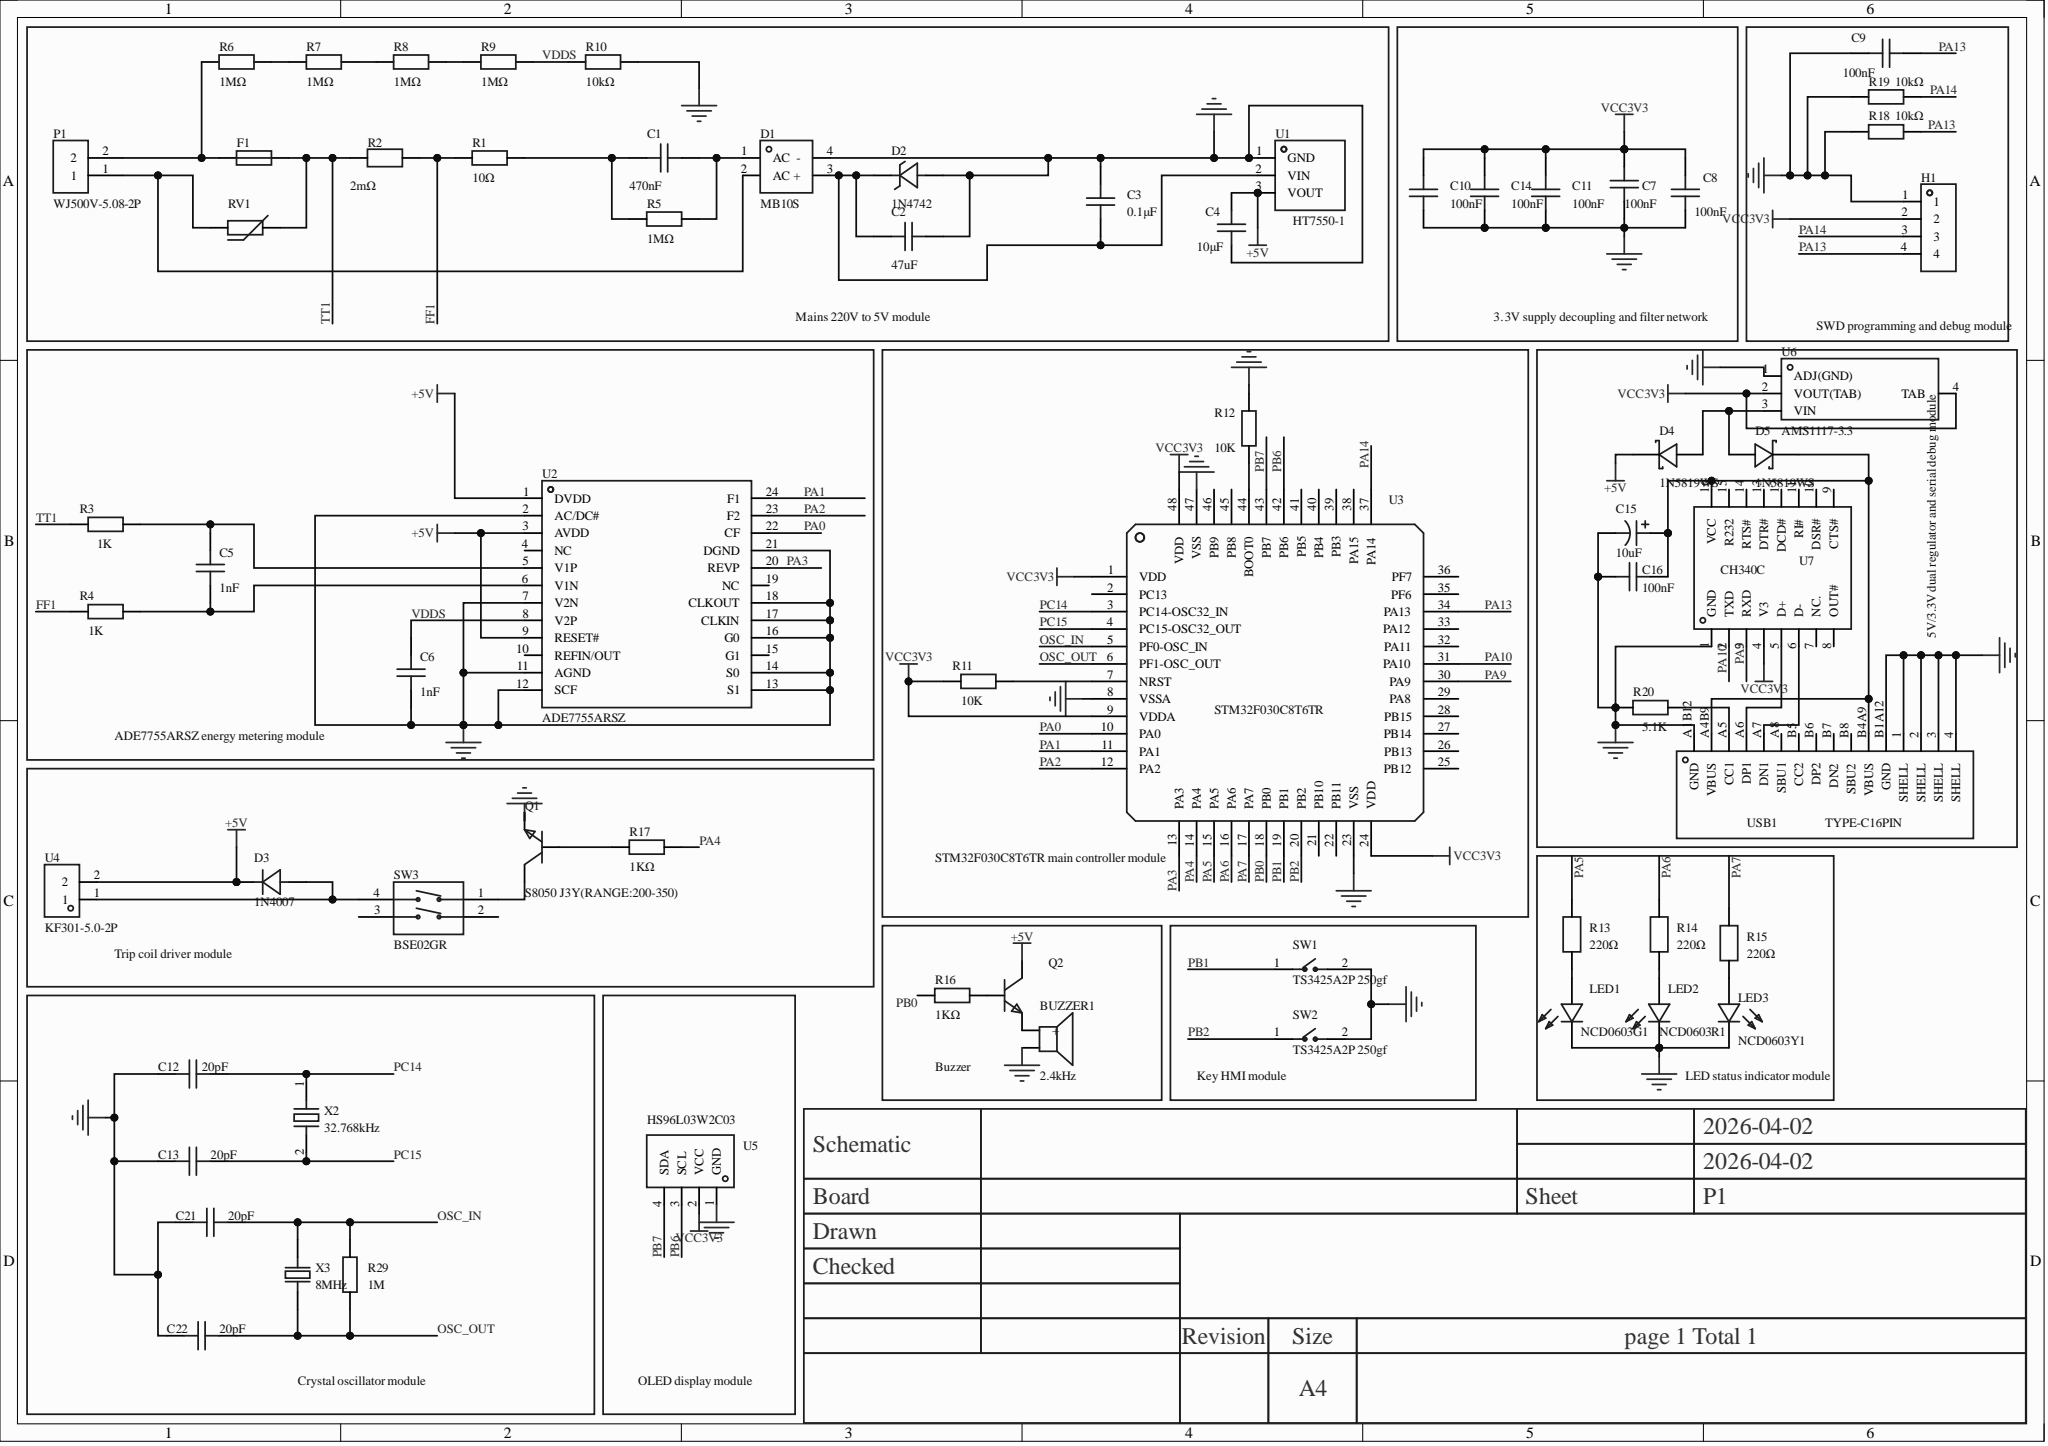Circuit board | Altium Designer | 67 parts | 52 nets
Bill of materials:
Comment,Description,Designator,Footprint,LibRef,Quantity
"2.4kHz","Drive method: Active (with built-in driver circuit); Construction type: Electromagnetic; Rated voltage: 5V; Frequency: 2.4kHz; Sound pressure (SPL): 85dB;","BUZZER1","BUZ-TH_BD12.0-P7.60-D0.6-FD","TMB12A05_C96093","1"
"470nF","Capacitance: 470nF; Tolerance: ±5%; Rated voltage: 400V; Operating temperature: -40℃~+105℃;","C1","CAP-TH_L17.0-W5.5-P15.00-D1.2","CBB21-400V474JP15","1"
"47uF","Capacitance: 47uF; Tolerance: ±20%; Rated voltage: 6.3V; Temperature coefficient: X5R;","C2","C0603","CL10A476MQ8QRNC","1"
"0.1µF","","C3","C0603","CAP_0603","1"
"10µF","","C4","C0603","CAP_0603","1"
"1nF","","C5, C6","C0603","CAP_0603","2"
"100nF","Capacitance: 100nF; Tolerance: ±10%; Rated voltage: 50V; Temperature coefficient: X7R;","C7, C8, C10, C14","C0805","GRM21BR71H104KA01L","4"
"100nF","Capacitance: 100nF; Tolerance: ±10%; Rated voltage: 50V; Temperature coefficient: X7R;, [NoValue]","C9, C11, C16","C0603","FCC0603B104K500CT, CAP_0603, CGA0603X7R104K500JT","3"
"20pF","","C12, C13, C21, C22","C0805","CAP_0805","4"
"10uF","Capacitance: 10uF; Tolerance: ±20%; Rated voltage: 50V; Ripple current: 24mA@120Hz; Equivalent series resistance (ESR): -;","C15","CAP-SMD_BD5.0-L5.3-W5.3-FD","RST10UF50V016","1"
"MB10S","Forward voltage (Vf): 1.1V@1A; DC reverse voltage (Vr): 1kV; Rectified current: 1A; Non-repetitive peak surge current (Ifsm): 35A;","D1","MBS_L4.7-W4.0-P2.50-LS7.0-TL","MB10S_C42463381","1"
"1N4742","Diode configuration: Single; Zener voltage (nominal): 12V; Zener voltage (range): 11.45V~12.95V; Power dissipation (Pd): 1W;","D2","DO-41_BD2.4-L4.7-P8.70-D0.8-FD","1N4742","1"
"1N4007","Diode configuration: Single; Forward voltage (Vf): 1.1V@1A; DC reverse voltage (Vr): 1kV; Rectified current: 1A;","D3","SMA_L4.3-W2.5-LS5.0-RD","1N4007_C727081","1"
"1N5819WS","Forward voltage (Vf): 600mV@1A; DC reverse voltage (Vr): 40V; Rectified current: 1A;","D4, D5","SOD-323_L1.8-W1.3-LS2.5-RD","1N5819WS_C191023","2"
"2F0.05002S1B02","Type: glass tube fuse; Rated current: 500mA; Rated voltage (AC): 250V; 125V; Breaking capacity: 50A;","F1","FUSE-TH_BD3.0-L7.2-P11.20-D0.6","2F0.05002S1B02","1"
"","","H1","HDR-TH_4P-P2.54-V-F","HDR-F_2.54_1x4P","1"
"NCD0603G1","Lamp head type: -; Emitting color: Emerald green; Forward voltage (Vf): 2.6V~3.6V; Power: 72mW; Forward current: 20mA; Wavelength: 515nm~530nm; Diode configuration: Single diode; Lens color: -; Color temperature: -; Luminous intensity: 900mcd; Viewing angle: 130°; Tape packing: -; Operating temperature: -30℃~+85℃;","LED1","LED0603-RD_1","NCD0603G1","1"
"NCD0603R1","Lamp head type: -; Emitting color: Red; Forward voltage (Vf): 1.6V~2.6V; Power: 65mW; Forward current: 25mA; Wavelength: 615nm~630nm; Diode configuration: Single diode; Lens color: -; Color temperature: -; Luminous intensity: 220mcd; Viewing angle: 130°; Tape packing: -; Operating temperature: -30℃~+85℃;","LED2","LED0603-RD_RED","NCD0603R1_C84263","1"
"NCD0603Y1","Lamp head type: -; Emitting color: Yellow; Forward voltage (Vf): 1.6V~2.6V; Power: 65mW; Forward current: 25mA; Wavelength: 586nm~595nm; Diode configuration: Single diode; Lens color: -; Color temperature: -; Luminous intensity: 220mcd; Viewing angle: 130°; Tape packing: -; Operating temperature: -30℃~+85℃;","LED3","LED0603-RD","NCD0603Y1","1"
"WJ500V-5.08-2P","Structure: 1x2P; Pitch: 5.08mm; Color: Green; Mounting: Through-hole; Rated current: 18A; Rated voltage: 250V; Rows: 1; Wire gauge - AWG: 14~30; Wire gauge - mm²: 2.5; Pins per row: 2; Contact material: -; Contact plating: -; Operating temperature range: -40℃~+105℃; Soldering temperature (max.): -;","P1","CONN-TH_2P-P5.00_WJ500V-5.08-2P","WJ500V-5.08-2P","1"
"S8050 J3Y(RANGE:200-350)","Transistor type: NPN; Collector current (Ic): 500mA; Collector-emitter breakdown voltage (Vceo): 25V; Power dissipation (Pd): 300mW; DC current gain (hFE): 200@500mA,1V;","Q1","SOT-23-3_L3.0-W1.7-P0.95-LS2.9-BR","S8050 J3Y(RANGE:200-350)","1"
"","","Q2","S8050_SOT-23","S8050_SOT_NPN","1"
"10Ω","","R1","R0603","Res_0603","1"
"2mΩ","Resistor type: Sense resistor; Resistance: 2mΩ; Tolerance: ±1%; Rated voltage drop: -; Power: 3W; Temperature coefficient: ±50ppm/?; Mounting: SMD;","R2","RES-SMD_L6.4-W3.2-1","HoLLR2512-3W-2mR-1%","1"
"1K","","R3, R4","R0603","Res_0603","2"
"1MΩ","","R5","R0603","Res_0603","1"
"1MΩ","Resistor type: Thick-film resistor; Resistance: 1MΩ; Tolerance: ±1%; Power: 250mW; Operating voltage: 200V; Temperature coefficient: ±100ppm/?;","R6, R7, R8, R9","R1206","1206W4F1004T5E","4"
"10kΩ","Resistor type: Thick-film resistor; Resistance: 10kΩ; Tolerance: ±1%; Power: 125mW; Operating voltage: 150V; Temperature coefficient: ±100ppm/?;","R10, R18, R19","R0805","0805W8F1002T5E_C17414","3"
"10K","","R11, R12","R0603","Res_0603","2"
"220Ω","Resistor type: Thick-film resistor; Resistance: 220Ω; Tolerance: ±1%; Power: 62.5mW; Operating voltage: 50V; Temperature coefficient: ±100ppm/?;","R13, R14, R15","R0402","FRC0402F2200TS","3"
"1KΩ","","R16, R17","R0603","Res_0603","2"
"5.1K","","R20","R0603","Res_0603","1"
"1M","","R29","R0805","Res_0805","1"
"190pF@1kHz","Varistor voltage: 423V~517V; Clamping voltage: 775V; Operating voltage (DC): 385V; Operating voltage (AC): 300V;","RV1","RES-TH_L12.5-W6.7-P7.50-D1.2","10D471K_C8760","1"
"TS3425A2P 250gf","Circuit structure: SPST; Button shape: Round; Actuation force: 2.5N; Mounting: Upright SMD; Length: 3.9mm; Width: 2.9mm; Height: 2.5mm; Bracket: No bracket; Contact current: 50mA; Rated voltage: 12V; Lamp: None; Operating life: 5 ten-thousand cycles;","SW1, SW2","SW-SMD_L3.9-W2.9-LS5.0","TS3425A2P 250gf","2"
"BSE02GR","Circuit structure: SPST; Number of positions: 2; Rated current: 25mA; Rated voltage: 24V; Operating life: 2 thousand cycles; Color: Red;","SW3","SW-TH_4P-L9.9-W6.8-P7.62-BL","BSE02GR","1"
"HT7550-1","Output type: Fixed; Operating voltage: 30V; Output voltage: 5V; Output current: 100mA; Power supply rejection ratio (PSRR): -; Output polarity: Positive;","U1","SOT-89_L4.5-W2.5-P1.50-LS4.2-BR","HT7550-1_C347189","1"
"ADE7755ARSZ","Operating voltage: 4.75V~5.25V; Operating current: 3.5mA;","U2","SSOP-24_L8.1-W5.3-P0.65-LS7.8-BL","ADE7755ARSZ","1"
"STM32F030C8T6TR","CPU core: ARM-M0; CPU max. frequency: 48MHz; Application field: -;","U3","LQFP-48_L7.0-W7.0-P0.50-LS9.0-BL","STM32F030C8T6TR","1"
"KF301-5.0-2P","Structure: 1x2P; Pitch: 5mm; Color: Blue; Mounting: Through-hole; Rows: 1; Pins per row: 2; Rated current: 17A; Rated voltage: 250V; Wire gauge - AWG: 14~22; Wire gauge - mm²: 1.5; Operating temperature: -30℃~+120℃;","U4","HDR-M-2.54_1X2","KF301-5.0-2P","1"
"HS96L03W2C03","Core chip: SSD1315 chip; Interface type: I2C; Size (inch): 0.96; Pixel resolution: 128x64;","U5","OLED-TH_L27.8-W27.2-P2.54_C9900033791","HS96L03W2C03","1"
"AMS1117-3.3","Output type: Fixed; Operating voltage: 12V; Output voltage: 3.3V; Output current: 1A; Power supply rejection ratio (PSRR): 60dB@(120Hz); Output polarity: Positive;","U6","SOT-223-4_L6.5-W3.5-P2.30-LS7.0-BR","AMS1117-3.3_C347222","1"
"CH340C","Application function: Transceiver; USB protocol version: USB 2.0; Data rate: 2Mbps;","U7","SOP-16_L10.0-W3.9-P1.27-LS6.0-BL","CH340C","1"
"TYPE-C16PIN","Connector type: Type-C; Protocol standard: -; Gender: Female; Mounting: Flat SMD; Contact count: 16P; Port count: 1; Rated current - power: 3A; Operating temperature: -40℃~+85℃;","USB1","USB-C-SMD_TYPE-C16PIN","TYPE-C16PIN","1"
"32.768kHz","Crystal type: SMD crystal; Frequency: 32.768kHz; Room-temperature frequency deviation: ±20ppm; Load capacitance: 20pF;","X2","CRYSTAL-SMD_L3.2-W1.5-FC-135R32.768KF-A3","7LC32768F06UC","1"
"8MHz","Crystal type: SMD crystal; Frequency: 8MHz; Room-temperature frequency deviation: ±10ppm; Load capacitance: 12pF; Frequency stability: ±20ppm;","X3","CRYSTAL-SMD_L3.2-W2.5_3225-8MHZ","X22EL89COI-111YLC-8M","1"
Netlist (Protel format):
[
BUZZER1
BUZ-TH_BD12.0-P7.60-D0.6-FD
2.4kHz



]
[
C1
CAP-TH_L17.0-W5.5-P15.00-D1.2
470nF



]
[
C2
C0603
47uF



]
[
C3
C0603
0.1µF



]
[
C4
C0603
10µF



]
[
C5
C0603
1nF



]
[
C6
C0603
1nF



]
[
C7
C0805
100nF



]
[
C8
C0805
100nF



]
[
C9
C0603
100nF



]
[
C10
C0805
100nF



]
[
C11
C0603
100nF



]
[
C12
C0805
20pF



]
[
C13
C0805
20pF



]
[
C14
C0805
100nF



]
[
C15
CAP-SMD_BD5.0-L5.3-W5.3-FD
10uF



]
[
C16
C0603
100nF



]
[
C21
C0805
20pF



]
[
C22
C0805
20pF



]
[
D1
MBS_L4.7-W4.0-P2.50-LS7.0-TL
MB10S



]
[
D2
DO-41_BD2.4-L4.7-P8.70-D0.8-FD
1N4742



]
[
D3
SMA_L4.3-W2.5-LS5.0-RD
1N4007



]
[
D4
SOD-323_L1.8-W1.3-LS2.5-RD
1N5819WS



]
[
D5
SOD-323_L1.8-W1.3-LS2.5-RD
1N5819WS



]
[
F1
FUSE-TH_BD3.0-L7.2-P11.20-D0.6
2F.0500212000S1B02



]
[
H1
HDR-TH_4P-P2.54-V-F




]
[
LED1
LED0603-RD_1
NCD0603G1



]
[
LED2
LED0603-RD_RED
NCD0603R1



]
[
LED3
LED0603-RD
NCD0603Y1



]
[
P1
CONN-TH_2P-P5.00_WJ500V-5.08-2P
WJ500V-5.08-2P



]
[
Q1
SOT-23-3_L3.0-W1.7-P0.95-LS2.9-BR
S8050 J3Y(RANGE:200-350)



]
[
Q2
S8050_SOT-23




]
[
R1
R0603
10Ω



]
[
R2
RES-SMD_L6.4-W3.2-1
2mΩ



]
[
R3
R0603
1K



]
[
R4
R0603
1K



]
[
R5
R0603
1MΩ



]
[
R6
R1206
1MΩ



]
[
R7
R1206
1MΩ



]
[
R8
R1206
1MΩ



]
[
R9
R1206
1MΩ



]
[
R10
R0805
10kΩ



]
[
R11
R0603
10K



]
[
R12
R0603
10K



]
[
R13
R0402
220Ω



]
[
R14
R0402
220Ω



]
[
R15
R0402
220Ω



]
[
R16
R0603
1KΩ



]
[
R17
R0603
1KΩ



]
[
R18
R0805
10kΩ



]
[
R19
R0805
10kΩ



]
[
R20
R0603
5.1K



]
[
R29
R0805
1M



]
[
RV1
RES-TH_L12.5-W6.7-P7.50-D1.2
190pF@1kHz



]
[
SW1
SW-SMD_L3.9-W2.9-LS5.0
TS3425A2P 250gf



]
[
SW2
SW-SMD_L3.9-W2.9-LS5.0
TS3425A2P 250gf



]
[
SW3
SW-TH_4P-L9.9-W6.8-P7.62-BL
BSE02GR



]
[
U1
SOT-89_L4.5-W2.5-P1.50-LS4.2-BR
HT7550-1



]
[
U2
SSOP-24_L8.1-W5.3-P0.65-LS7.8-BL
ADE7755ARSZ



]
[
U3
LQFP-48_L7.0-W7.0-P0.50-LS9.0-BL
STM32F030C8T6TR



]
[
U4
HDR-M-2.54_1X2
KF301-5.0-2P



]
[
U5
OLED-TH_L27.8-W27.2-P2.54_C9900033791
HS96L03W2C03



]
[
U6
SOT-223-4_L6.5-W3.5-P2.30-LS7.0-BR
AMS1117-3.3



]
[
U7
SOP-16_L10.0-W3.9-P1.27-LS6.0-BL
CH340C



]
[
USB1
USB-C-SMD_TYPE-C16PIN
TYPE-C16PIN



]
[
X2
CRYSTAL-SMD_L3.2-W1.5-FC-135R32.7680KF-A3
32.768kHz



]
[
X3
CRYSTAL-SMD_L3.2-W2.5_3225-8MHZ
8MHz



]
(
VDDS
C6-2
R9-2
R10-1
U2-8
)
(
VCC3V3
C7-1
C8-2
C10-1
C11-2
C14-2
H1-2
R11-1
U3-1
U3-9
U3-24
U3-48
U5-2
U6-2
U6-4
U7-4
)
(
TT1
F1-2
R2-1
R3-1
RV1-2
)
(
PC15
C13-2
U3-4
X2-2
)
(
PC14
C12-1
U3-3
X2-1
)
(
PB7
U3-43
U5-4
)
(
PB6
U3-42
U5-3
)
(
PB2
SW2-1
U3-20
)
(
PB1
SW1-1
U3-19
)
(
PB0
R16-2
U3-18
)
(
PA14
H1-3
R19-1
U3-37
)
(
PA13
C9-2
H1-4
R18-1
U3-34
)
(
PA10
U3-31
U7-2
)
(
PA9
U3-30
U7-3
)
(
PA7
R15-2
U3-17
)
(
PA6
R14-2
U3-16
)
(
PA5
R13-2
U3-15
)
(
PA4
R17-1
U3-14
)
(
PA3
U2-20
U3-13
)
(
PA2
U2-23
U3-12
)
(
PA1
U2-24
U3-11
)
(
PA0
U2-22
U3-10
)
(
OSC_OUT
C22-2
R29-1
U3-6
X3-1
)
(
OSC_IN
C21-2
R29-2
U3-5
X3-2
)
(
NetU7_6
U7-6
USB1-A7
)
(
NetU7_5
U7-5
USB1-A6
)
(
NetR20_1
R20-1
USB1-A5
)
(
NetR12_1
R12-1
U3-44
)
(
NetR11_2
R11-2
U3-7
)
(
NetR8_2
R8-2
R9-1
)
(
NetR7_2
R7-2
R8-1
)
(
NetR6_2
R6-2
R7-1
)
(
NetQ2_1
Q2-1
R16-1
)
(
NetQ1_3
Q1-3
SW3-1
)
(
NetQ1_1
Q1-1
R17-2
)
(
NetLED3_2
LED3-2
R15-1
)
(
NetLED2_2
LED2-2
R14-1
)
(
NetLED1_2
LED1-2
R13-1
)
(
NetF1_1
F1-1
P1-2
R6-1
)
(
NetD4_2
D4-2
D5-2
U6-3
)
(
NetD3_2
D3-2
SW3-4
U4-1
)
(
NetD1_2
D1-2
P1-1
RV1-1
)
(
NetC15_1
C15-1
C16-2
D5-1
U7-16
USB1-A4B9
USB1-B4A9
)
(
NetC5_2
C5-2
R3-2
U2-5
)
(
NetC5_1
C5-1
R4-2
U2-6
)
(
NetC2_1
C2-1
C3-1
D1-3
D2-2
U1-2
)
(
NetC1_2
C1-2
R1-2
R5-1
)
(
NetC1_1
C1-1
D1-1
R5-2
)
(
NetBUZZER1_1
BUZZER1-1
Q2-2
)
(
GND
BUZZER1-2
C2-2
C3-2
C4-1
C6-1
C7-2
C8-1
C9-1
C10-2
C11-1
C12-2
C13-1
C14-1
C15-2
C16-1
C21-1
C22-1
D1-4
D2-1
H1-1
LED1-1
LED2-1
LED3-1
Q1-2
R10-2
R12-2
R18-2
R19-2
R20-2
SW1-2
SW2-2
U1-1
U2-2
U2-7
U2-11
U2-12
U2-13
U2-14
U2-16
U2-17
U2-18
U2-21
U3-8
U3-23
U3-47
U5-1
U6-1
U7-1
USB1-1
USB1-2
USB1-3
USB1-4
USB1-A1B12
USB1-B1A12
)
(
FF1
R1-1
R2-2
R4-1
)
(
+5V
C4-2
D3-1
D4-1
Q2-3
U1-3
U2-1
U2-3
U2-9
U4-2
)